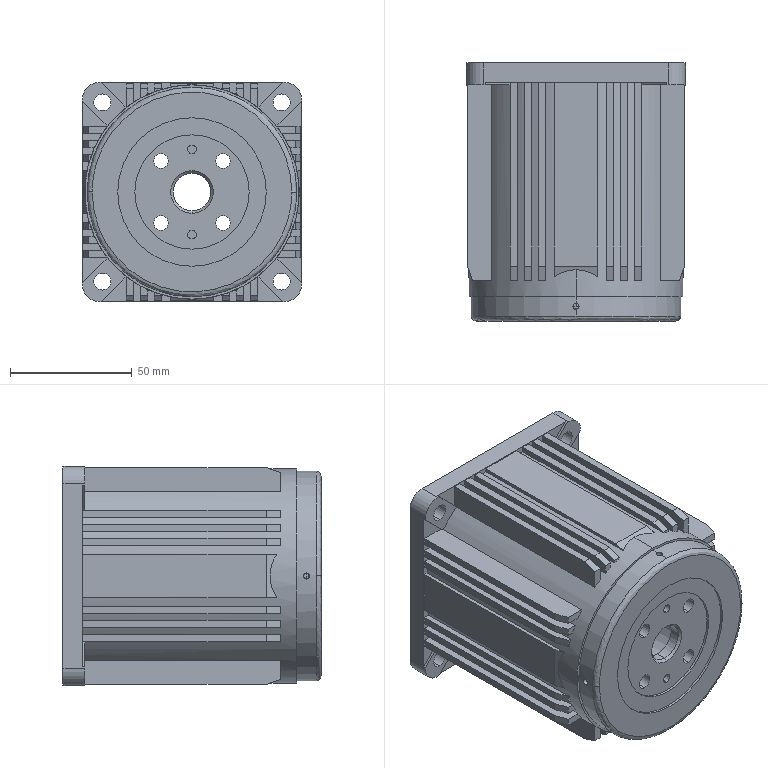Part | STEP file | 1 solid | 263 faces | box 90 x 106 x 90 mm | volume 163819 mm3 | plane 174 | cylinder 79 | cone 8 | spline 2 | commonest cylinder face diameters 9 x15 2.5 x8 6.1 x8 7 x8 33 x8 3.6 x4